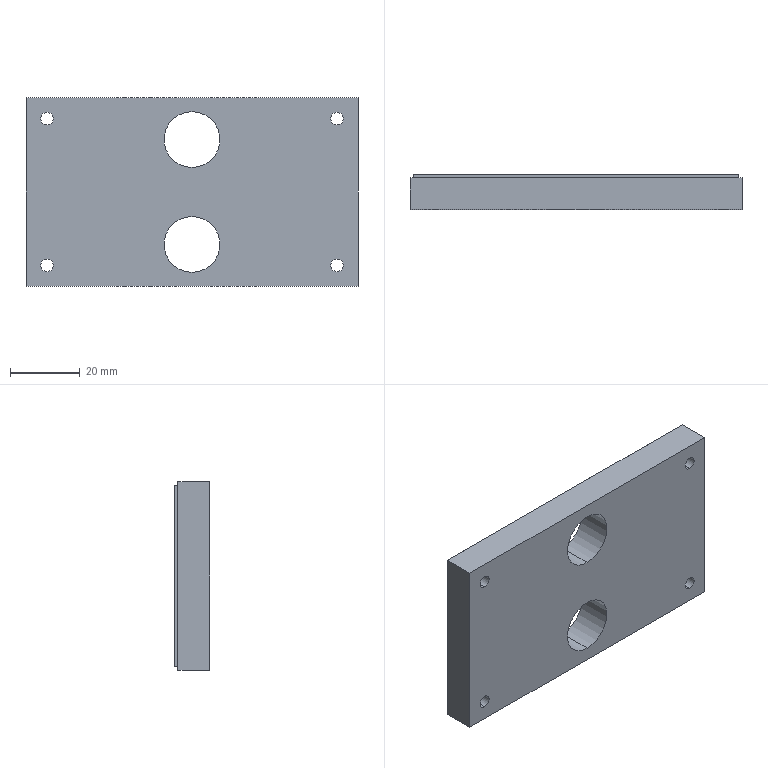Part | SolidWorks | features ICE 2, 3DProfileFeature 1, Chamfer 1, Extrusion 1, HoleWzd 1 | 1 solid | 43 faces | box 95 x 10.05 x 54 mm | volume 46492 mm3 | cylinder 20 | plane 15 | cone 8 | commonest cylinder face diameters 3.6 x8 7 x8 16 x4
STEP:
#1=CARTESIAN_POINT('',(47.5,0.,-4.));
#2=VERTEX_POINT('',#1);
#3=CARTESIAN_POINT('',(47.5,0.,-20.));
#4=VERTEX_POINT('',#3);
#5=CARTESIAN_POINT('',(47.5,0.,-12.));
#6=DIRECTION('',(0.,-1.,0.));
#7=DIRECTION('',(0.,0.,-1.));
#8=AXIS2_PLACEMENT_3D('',#5,#6,#7);
#9=CIRCLE('',#8,8.);
#10=EDGE_CURVE('',#2,#4,#9,.T.);
#11=ORIENTED_EDGE('',*,*,#10,.T.);
#12=CARTESIAN_POINT('',(47.5,10.05,-20.));
#13=VERTEX_POINT('',#12);
#14=CARTESIAN_POINT('',(47.5,-0.001,-20.));
#15=DIRECTION('',(0.,1.,0.));
#16=VECTOR('',#15,1000.);
#17=LINE('',#14,#16);
#18=EDGE_CURVE('',#4,#13,#17,.T.);
#19=ORIENTED_EDGE('',*,*,#18,.T.);
#20=CARTESIAN_POINT('',(47.5,10.05,-4.));
#21=VERTEX_POINT('',#20);
#22=CARTESIAN_POINT('',(47.5,10.05,-12.));
#23=DIRECTION('',(0.,-1.,0.));
#24=DIRECTION('',(0.,0.,1.));
#25=AXIS2_PLACEMENT_3D('',#22,#23,#24);
#26=CIRCLE('',#25,8.);
#27=EDGE_CURVE('',#21,#13,#26,.T.);
#28=ORIENTED_EDGE('',*,*,#27,.F.);
#29=CARTESIAN_POINT('',(47.5,-0.001,-4.));
#30=DIRECTION('',(0.,1.,0.));
#31=VECTOR('',#30,1000.);
#32=LINE('',#29,#31);
#33=EDGE_CURVE('',#2,#21,#32,.T.);
#34=ORIENTED_EDGE('',*,*,#33,.F.);
#35=EDGE_LOOP('',(#11,#19,#28,#34));
#36=FACE_OUTER_BOUND('',#35,.T.);
#37=CARTESIAN_POINT('',(47.5,-0.001,-12.));
#38=DIRECTION('',(0.,1.,0.));
#39=DIRECTION('',(0.,0.,1.));
#40=AXIS2_PLACEMENT_3D('',#37,#38,#39);
#41=CYLINDRICAL_SURFACE('',#40,8.);
#42=ADVANCED_FACE('',(#36),#41,.F.);
#43=CARTESIAN_POINT('',(47.5,0.,-50.));
#44=VERTEX_POINT('',#43);
#45=CARTESIAN_POINT('',(47.5,0.,-34.));
#46=VERTEX_POINT('',#45);
#47=CARTESIAN_POINT('',(47.5,0.,-42.));
#48=DIRECTION('',(0.,1.,0.));
#49=DIRECTION('',(0.,0.,-1.));
#50=AXIS2_PLACEMENT_3D('',#47,#48,#49);
#51=CIRCLE('',#50,8.);
#52=EDGE_CURVE('',#44,#46,#51,.T.);
#53=ORIENTED_EDGE('',*,*,#52,.F.);
#54=CARTESIAN_POINT('',(47.5,10.05,-50.));
#55=VERTEX_POINT('',#54);
#56=CARTESIAN_POINT('',(47.5,-0.001,-50.));
#57=DIRECTION('',(0.,1.,0.));
#58=VECTOR('',#57,1000.);
#59=LINE('',#56,#58);
#60=EDGE_CURVE('',#44,#55,#59,.T.);
#61=ORIENTED_EDGE('',*,*,#60,.T.);
#62=CARTESIAN_POINT('',(47.5,10.05,-34.));
#63=VERTEX_POINT('',#62);
#64=CARTESIAN_POINT('',(47.5,10.05,-42.));
#65=DIRECTION('',(0.,1.,0.));
#66=DIRECTION('',(0.,0.,1.));
#67=AXIS2_PLACEMENT_3D('',#64,#65,#66);
#68=CIRCLE('',#67,8.);
#69=EDGE_CURVE('',#55,#63,#68,.T.);
#70=ORIENTED_EDGE('',*,*,#69,.T.);
#71=CARTESIAN_POINT('',(47.5,-0.001,-34.));
#72=DIRECTION('',(0.,1.,0.));
#73=VECTOR('',#72,1000.);
#74=LINE('',#71,#73);
#75=EDGE_CURVE('',#46,#63,#74,.T.);
#76=ORIENTED_EDGE('',*,*,#75,.F.);
#77=EDGE_LOOP('',(#53,#61,#70,#76));
#78=FACE_OUTER_BOUND('',#77,.T.);
#79=CARTESIAN_POINT('',(47.5,-0.001,-42.));
#80=DIRECTION('',(0.,1.,0.));
#81=DIRECTION('',(0.,0.,1.));
#82=AXIS2_PLACEMENT_3D('',#79,#80,#81);
#83=CYLINDRICAL_SURFACE('',#82,8.);
#84=ADVANCED_FACE('',(#78),#83,.F.);
#85=CARTESIAN_POINT('',(6.,9.05,-51.5));
#86=VERTEX_POINT('',#85);
#87=CARTESIAN_POINT('',(6.,9.05,-44.5));
#88=VERTEX_POINT('',#87);
#89=CARTESIAN_POINT('',(6.,9.05,-48.));
#90=DIRECTION('',(0.,1.,0.));
#91=DIRECTION('',(0.,0.,-1.));
#92=AXIS2_PLACEMENT_3D('',#89,#90,#91);
#93=CIRCLE('',#92,3.5);
#94=EDGE_CURVE('',#86,#88,#93,.T.);
#95=ORIENTED_EDGE('',*,*,#94,.F.);
#96=CARTESIAN_POINT('',(6.,10.05,-52.5));
#97=VERTEX_POINT('',#96);
#98=CARTESIAN_POINT('',(6.,9.05,-51.5));
#99=DIRECTION('',(0.,0.7071,-0.7071));
#100=VECTOR('',#99,1000.);
#101=LINE('',#98,#100);
#102=EDGE_CURVE('',#86,#97,#101,.T.);
#103=ORIENTED_EDGE('',*,*,#102,.T.);
#104=CARTESIAN_POINT('',(6.,10.05,-43.5));
#105=VERTEX_POINT('',#104);
#106=CARTESIAN_POINT('',(6.,10.05,-48.));
#107=DIRECTION('',(0.,-1.,0.));
#108=DIRECTION('',(0.,0.,-1.));
#109=AXIS2_PLACEMENT_3D('',#106,#107,#108);
#110=CIRCLE('',#109,4.5);
#111=EDGE_CURVE('',#105,#97,#110,.T.);
#112=ORIENTED_EDGE('',*,*,#111,.F.);
#113=CARTESIAN_POINT('',(6.,9.05,-44.5));
#114=DIRECTION('',(0.,0.7071,0.7071));
#115=VECTOR('',#114,1000.);
#116=LINE('',#113,#115);
#117=EDGE_CURVE('',#88,#105,#116,.T.);
#118=ORIENTED_EDGE('',*,*,#117,.F.);
#119=EDGE_LOOP('',(#95,#103,#112,#118));
#120=FACE_OUTER_BOUND('',#119,.T.);
#121=CARTESIAN_POINT('',(6.,9.05,-48.));
#122=DIRECTION('',(0.,1.,0.));
#123=DIRECTION('',(0.,0.,1.));
#124=AXIS2_PLACEMENT_3D('',#121,#122,#123);
#125=CONICAL_SURFACE('',#124,3.5,0.7854);
#126=ADVANCED_FACE('',(#120),#125,.F.);
#127=CARTESIAN_POINT('',(6.,9.05,-9.5));
#128=VERTEX_POINT('',#127);
#129=CARTESIAN_POINT('',(6.,9.05,-2.5));
#130=VERTEX_POINT('',#129);
#131=CARTESIAN_POINT('',(6.,9.05,-6.));
#132=DIRECTION('',(0.,1.,0.));
#133=DIRECTION('',(0.,0.,-1.));
#134=AXIS2_PLACEMENT_3D('',#131,#132,#133);
#135=CIRCLE('',#134,3.5);
#136=EDGE_CURVE('',#128,#130,#135,.T.);
#137=ORIENTED_EDGE('',*,*,#136,.F.);
#138=CARTESIAN_POINT('',(6.,10.05,-10.5));
#139=VERTEX_POINT('',#138);
#140=CARTESIAN_POINT('',(6.,9.05,-9.5));
#141=DIRECTION('',(0.,0.7071,-0.7071));
#142=VECTOR('',#141,1000.);
#143=LINE('',#140,#142);
#144=EDGE_CURVE('',#128,#139,#143,.T.);
#145=ORIENTED_EDGE('',*,*,#144,.T.);
#146=CARTESIAN_POINT('',(6.,10.05,-1.5));
#147=VERTEX_POINT('',#146);
#148=CARTESIAN_POINT('',(6.,10.05,-6.));
#149=DIRECTION('',(0.,-1.,0.));
#150=DIRECTION('',(0.,0.,-1.));
#151=AXIS2_PLACEMENT_3D('',#148,#149,#150);
#152=CIRCLE('',#151,4.5);
#153=EDGE_CURVE('',#147,#139,#152,.T.);
#154=ORIENTED_EDGE('',*,*,#153,.F.);
#155=CARTESIAN_POINT('',(6.,9.05,-2.5));
#156=DIRECTION('',(0.,0.7071,0.7071));
#157=VECTOR('',#156,1000.);
#158=LINE('',#155,#157);
#159=EDGE_CURVE('',#130,#147,#158,.T.);
#160=ORIENTED_EDGE('',*,*,#159,.F.);
#161=EDGE_LOOP('',(#137,#145,#154,#160));
#162=FACE_OUTER_BOUND('',#161,.T.);
#163=CARTESIAN_POINT('',(6.,9.05,-6.));
#164=DIRECTION('',(0.,1.,0.));
#165=DIRECTION('',(0.,0.,1.));
#166=AXIS2_PLACEMENT_3D('',#163,#164,#165);
#167=CONICAL_SURFACE('',#166,3.5,0.7854);
#168=ADVANCED_FACE('',(#162),#167,.F.);
#169=CARTESIAN_POINT('',(89.,9.05,-51.5));
#170=VERTEX_POINT('',#169);
#171=CARTESIAN_POINT('',(89.,9.05,-44.5));
#172=VERTEX_POINT('',#171);
#173=CARTESIAN_POINT('',(89.,9.05,-48.));
#174=DIRECTION('',(0.,1.,0.));
#175=DIRECTION('',(0.,0.,-1.));
#176=AXIS2_PLACEMENT_3D('',#173,#174,#175);
#177=CIRCLE('',#176,3.5);
#178=EDGE_CURVE('',#170,#172,#177,.T.);
#179=ORIENTED_EDGE('',*,*,#178,.F.);
#180=CARTESIAN_POINT('',(89.,10.05,-52.5));
#181=VERTEX_POINT('',#180);
#182=CARTESIAN_POINT('',(89.,9.05,-51.5));
#183=DIRECTION('',(0.,0.7071,-0.7071));
#184=VECTOR('',#183,1000.);
#185=LINE('',#182,#184);
#186=EDGE_CURVE('',#170,#181,#185,.T.);
#187=ORIENTED_EDGE('',*,*,#186,.T.);
#188=CARTESIAN_POINT('',(89.,10.05,-43.5));
#189=VERTEX_POINT('',#188);
#190=CARTESIAN_POINT('',(89.,10.05,-48.));
#191=DIRECTION('',(0.,-1.,0.));
#192=DIRECTION('',(0.,0.,-1.));
#193=AXIS2_PLACEMENT_3D('',#190,#191,#192);
#194=CIRCLE('',#193,4.5);
#195=EDGE_CURVE('',#189,#181,#194,.T.);
#196=ORIENTED_EDGE('',*,*,#195,.F.);
#197=CARTESIAN_POINT('',(89.,9.05,-44.5));
#198=DIRECTION('',(0.,0.7071,0.7071));
#199=VECTOR('',#198,1000.);
#200=LINE('',#197,#199);
#201=EDGE_CURVE('',#172,#189,#200,.T.);
#202=ORIENTED_EDGE('',*,*,#201,.F.);
#203=EDGE_LOOP('',(#179,#187,#196,#202));
#204=FACE_OUTER_BOUND('',#203,.T.);
#205=CARTESIAN_POINT('',(89.,9.05,-48.));
#206=DIRECTION('',(0.,1.,0.));
#207=DIRECTION('',(0.,0.,1.));
#208=AXIS2_PLACEMENT_3D('',#205,#206,#207);
#209=CONICAL_SURFACE('',#208,3.5,0.7854);
#210=ADVANCED_FACE('',(#204),#209,.F.);
#211=CARTESIAN_POINT('',(89.,9.05,-9.5));
#212=VERTEX_POINT('',#211);
#213=CARTESIAN_POINT('',(89.,9.05,-2.5));
#214=VERTEX_POINT('',#213);
#215=CARTESIAN_POINT('',(89.,9.05,-6.));
#216=DIRECTION('',(0.,1.,0.));
#217=DIRECTION('',(0.,0.,-1.));
#218=AXIS2_PLACEMENT_3D('',#215,#216,#217);
#219=CIRCLE('',#218,3.5);
#220=EDGE_CURVE('',#212,#214,#219,.T.);
#221=ORIENTED_EDGE('',*,*,#220,.F.);
#222=CARTESIAN_POINT('',(89.,10.05,-10.5));
#223=VERTEX_POINT('',#222);
#224=CARTESIAN_POINT('',(89.,9.05,-9.5));
#225=DIRECTION('',(0.,0.7071,-0.7071));
#226=VECTOR('',#225,1000.);
#227=LINE('',#224,#226);
#228=EDGE_CURVE('',#212,#223,#227,.T.);
#229=ORIENTED_EDGE('',*,*,#228,.T.);
#230=CARTESIAN_POINT('',(89.,10.05,-1.5));
#231=VERTEX_POINT('',#230);
#232=CARTESIAN_POINT('',(89.,10.05,-6.));
#233=DIRECTION('',(0.,-1.,0.));
#234=DIRECTION('',(0.,0.,-1.));
#235=AXIS2_PLACEMENT_3D('',#232,#233,#234);
#236=CIRCLE('',#235,4.5);
#237=EDGE_CURVE('',#231,#223,#236,.T.);
#238=ORIENTED_EDGE('',*,*,#237,.F.);
#239=CARTESIAN_POINT('',(89.,9.05,-2.5));
#240=DIRECTION('',(0.,0.7071,0.7071));
#241=VECTOR('',#240,1000.);
#242=LINE('',#239,#241);
#243=EDGE_CURVE('',#214,#231,#242,.T.);
#244=ORIENTED_EDGE('',*,*,#243,.F.);
#245=EDGE_LOOP('',(#221,#229,#238,#244));
#246=FACE_OUTER_BOUND('',#245,.T.);
#247=CARTESIAN_POINT('',(89.,9.05,-6.));
#248=DIRECTION('',(0.,1.,0.));
#249=DIRECTION('',(0.,0.,1.));
#250=AXIS2_PLACEMENT_3D('',#247,#248,#249);
#251=CONICAL_SURFACE('',#250,3.5,0.7854);
#252=ADVANCED_FACE('',(#246),#251,.F.);
#253=CARTESIAN_POINT('',(6.,7.65,-51.5));
#254=VERTEX_POINT('',#253);
#255=CARTESIAN_POINT('',(6.,7.65,-44.5));
#256=VERTEX_POINT('',#255);
#257=CARTESIAN_POINT('',(6.,7.65,-48.));
#258=DIRECTION('',(0.,1.,0.));
#259=DIRECTION('',(0.,0.,1.));
#260=AXIS2_PLACEMENT_3D('',#257,#258,#259);
#261=CIRCLE('',#260,3.5);
#262=EDGE_CURVE('',#254,#256,#261,.T.);
#263=ORIENTED_EDGE('',*,*,#262,.F.);
#264=CARTESIAN_POINT('',(6.,10.05,-51.5));
#265=DIRECTION('',(0.,1.,0.));
#266=VECTOR('',#265,1000.);
#267=LINE('',#264,#266);
#268=EDGE_CURVE('',#254,#86,#267,.T.);
#269=ORIENTED_EDGE('',*,*,#268,.T.);
#270=ORIENTED_EDGE('',*,*,#94,.T.);
#271=CARTESIAN_POINT('',(6.,10.05,-44.5));
#272=DIRECTION('',(0.,1.,0.));
#273=VECTOR('',#272,1000.);
#274=LINE('',#271,#273);
#275=EDGE_CURVE('',#256,#88,#274,.T.);
#276=ORIENTED_EDGE('',*,*,#275,.F.);
#277=EDGE_LOOP('',(#263,#269,#270,#276));
#278=FACE_OUTER_BOUND('',#277,.T.);
#279=CARTESIAN_POINT('',(6.,10.05,-48.));
#280=DIRECTION('',(0.,1.,0.));
#281=DIRECTION('',(0.,0.,1.));
#282=AXIS2_PLACEMENT_3D('',#279,#280,#281);
#283=CYLINDRICAL_SURFACE('',#282,3.5);
#284=ADVANCED_FACE('',(#278),#283,.F.);
#285=CARTESIAN_POINT('',(6.,0.,-46.2));
#286=VERTEX_POINT('',#285);
#287=CARTESIAN_POINT('',(6.,0.,-49.8));
#288=VERTEX_POINT('',#287);
#289=CARTESIAN_POINT('',(6.,0.,-48.));
#290=DIRECTION('',(0.,-1.,0.));
#291=DIRECTION('',(0.,0.,-1.));
#292=AXIS2_PLACEMENT_3D('',#289,#290,#291);
#293=CIRCLE('',#292,1.8);
#294=EDGE_CURVE('',#286,#288,#293,.T.);
#295=ORIENTED_EDGE('',*,*,#294,.T.);
#296=CARTESIAN_POINT('',(6.,7.65,-49.8));
#297=VERTEX_POINT('',#296);
#298=CARTESIAN_POINT('',(6.,10.05,-49.8));
#299=DIRECTION('',(0.,1.,0.));
#300=VECTOR('',#299,1000.);
#301=LINE('',#298,#300);
#302=EDGE_CURVE('',#288,#297,#301,.T.);
#303=ORIENTED_EDGE('',*,*,#302,.T.);
#304=CARTESIAN_POINT('',(6.,7.65,-46.2));
#305=VERTEX_POINT('',#304);
#306=CARTESIAN_POINT('',(6.,7.65,-48.));
#307=DIRECTION('',(0.,1.,0.));
#308=DIRECTION('',(0.,0.,1.));
#309=AXIS2_PLACEMENT_3D('',#306,#307,#308);
#310=CIRCLE('',#309,1.8);
#311=EDGE_CURVE('',#297,#305,#310,.T.);
#312=ORIENTED_EDGE('',*,*,#311,.T.);
#313=CARTESIAN_POINT('',(6.,10.05,-46.2));
#314=DIRECTION('',(0.,1.,0.));
#315=VECTOR('',#314,1000.);
#316=LINE('',#313,#315);
#317=EDGE_CURVE('',#286,#305,#316,.T.);
#318=ORIENTED_EDGE('',*,*,#317,.F.);
#319=EDGE_LOOP('',(#295,#303,#312,#318));
#320=FACE_OUTER_BOUND('',#319,.T.);
#321=CARTESIAN_POINT('',(6.,10.05,-48.));
#322=DIRECTION('',(0.,1.,0.));
#323=DIRECTION('',(0.,0.,1.));
#324=AXIS2_PLACEMENT_3D('',#321,#322,#323);
#325=CYLINDRICAL_SURFACE('',#324,1.8);
#326=ADVANCED_FACE('',(#320),#325,.F.);
#327=CARTESIAN_POINT('',(89.,7.65,-51.5));
#328=VERTEX_POINT('',#327);
#329=CARTESIAN_POINT('',(89.,7.65,-44.5));
#330=VERTEX_POINT('',#329);
#331=CARTESIAN_POINT('',(89.,7.65,-48.));
#332=DIRECTION('',(0.,1.,0.));
#333=DIRECTION('',(0.,0.,1.));
#334=AXIS2_PLACEMENT_3D('',#331,#332,#333);
#335=CIRCLE('',#334,3.5);
#336=EDGE_CURVE('',#328,#330,#335,.T.);
#337=ORIENTED_EDGE('',*,*,#336,.F.);
#338=CARTESIAN_POINT('',(89.,10.05,-51.5));
#339=DIRECTION('',(0.,1.,0.));
#340=VECTOR('',#339,1000.);
#341=LINE('',#338,#340);
#342=EDGE_CURVE('',#328,#170,#341,.T.);
#343=ORIENTED_EDGE('',*,*,#342,.T.);
#344=ORIENTED_EDGE('',*,*,#178,.T.);
#345=CARTESIAN_POINT('',(89.,10.05,-44.5));
#346=DIRECTION('',(0.,1.,0.));
#347=VECTOR('',#346,1000.);
#348=LINE('',#345,#347);
#349=EDGE_CURVE('',#330,#172,#348,.T.);
#350=ORIENTED_EDGE('',*,*,#349,.F.);
#351=EDGE_LOOP('',(#337,#343,#344,#350));
#352=FACE_OUTER_BOUND('',#351,.T.);
#353=CARTESIAN_POINT('',(89.,10.05,-48.));
#354=DIRECTION('',(0.,1.,0.));
#355=DIRECTION('',(0.,0.,1.));
#356=AXIS2_PLACEMENT_3D('',#353,#354,#355);
#357=CYLINDRICAL_SURFACE('',#356,3.5);
#358=ADVANCED_FACE('',(#352),#357,.F.);
#359=CARTESIAN_POINT('',(89.,0.,-46.2));
#360=VERTEX_POINT('',#359);
#361=CARTESIAN_POINT('',(89.,0.,-49.8));
#362=VERTEX_POINT('',#361);
#363=CARTESIAN_POINT('',(89.,0.,-48.));
#364=DIRECTION('',(0.,-1.,0.));
#365=DIRECTION('',(0.,0.,-1.));
#366=AXIS2_PLACEMENT_3D('',#363,#364,#365);
#367=CIRCLE('',#366,1.8);
#368=EDGE_CURVE('',#360,#362,#367,.T.);
#369=ORIENTED_EDGE('',*,*,#368,.T.);
#370=CARTESIAN_POINT('',(89.,7.65,-49.8));
#371=VERTEX_POINT('',#370);
#372=CARTESIAN_POINT('',(89.,10.05,-49.8));
#373=DIRECTION('',(0.,1.,0.));
#374=VECTOR('',#373,1000.);
#375=LINE('',#372,#374);
#376=EDGE_CURVE('',#362,#371,#375,.T.);
#377=ORIENTED_EDGE('',*,*,#376,.T.);
#378=CARTESIAN_POINT('',(89.,7.65,-46.2));
#379=VERTEX_POINT('',#378);
#380=CARTESIAN_POINT('',(89.,7.65,-48.));
#381=DIRECTION('',(0.,1.,0.));
#382=DIRECTION('',(0.,0.,1.));
#383=AXIS2_PLACEMENT_3D('',#380,#381,#382);
#384=CIRCLE('',#383,1.8);
#385=EDGE_CURVE('',#371,#379,#384,.T.);
#386=ORIENTED_EDGE('',*,*,#385,.T.);
#387=CARTESIAN_POINT('',(89.,10.05,-46.2));
#388=DIRECTION('',(0.,1.,0.));
#389=VECTOR('',#388,1000.);
#390=LINE('',#387,#389);
#391=EDGE_CURVE('',#360,#379,#390,.T.);
#392=ORIENTED_EDGE('',*,*,#391,.F.);
#393=EDGE_LOOP('',(#369,#377,#386,#392));
#394=FACE_OUTER_BOUND('',#393,.T.);
#395=CARTESIAN_POINT('',(89.,10.05,-48.));
#396=DIRECTION('',(0.,1.,0.));
#397=DIRECTION('',(0.,0.,1.));
#398=AXIS2_PLACEMENT_3D('',#395,#396,#397);
#399=CYLINDRICAL_SURFACE('',#398,1.8);
#400=ADVANCED_FACE('',(#394),#399,.F.);
#401=CARTESIAN_POINT('',(89.,7.65,-9.5));
#402=VERTEX_POINT('',#401);
#403=CARTESIAN_POINT('',(89.,7.65,-2.5));
#404=VERTEX_POINT('',#403);
#405=CARTESIAN_POINT('',(89.,7.65,-6.));
#406=DIRECTION('',(0.,1.,0.));
#407=DIRECTION('',(0.,0.,1.));
#408=AXIS2_PLACEMENT_3D('',#405,#406,#407);
#409=CIRCLE('',#408,3.5);
#410=EDGE_CURVE('',#402,#404,#409,.T.);
#411=ORIENTED_EDGE('',*,*,#410,.F.);
#412=CARTESIAN_POINT('',(89.,10.05,-9.5));
#413=DIRECTION('',(0.,1.,0.));
#414=VECTOR('',#413,1000.);
#415=LINE('',#412,#414);
#416=EDGE_CURVE('',#402,#212,#415,.T.);
#417=ORIENTED_EDGE('',*,*,#416,.T.);
#418=ORIENTED_EDGE('',*,*,#220,.T.);
#419=CARTESIAN_POINT('',(89.,10.05,-2.5));
#420=DIRECTION('',(0.,1.,0.));
#421=VECTOR('',#420,1000.);
#422=LINE('',#419,#421);
#423=EDGE_CURVE('',#404,#214,#422,.T.);
#424=ORIENTED_EDGE('',*,*,#423,.F.);
#425=EDGE_LOOP('',(#411,#417,#418,#424));
#426=FACE_OUTER_BOUND('',#425,.T.);
#427=CARTESIAN_POINT('',(89.,10.05,-6.));
#428=DIRECTION('',(0.,1.,0.));
#429=DIRECTION('',(0.,0.,1.));
#430=AXIS2_PLACEMENT_3D('',#427,#428,#429);
#431=CYLINDRICAL_SURFACE('',#430,3.5);
#432=ADVANCED_FACE('',(#426),#431,.F.);
#433=CARTESIAN_POINT('',(89.,0.,-4.2));
#434=VERTEX_POINT('',#433);
#435=CARTESIAN_POINT('',(89.,0.,-7.8));
#436=VERTEX_POINT('',#435);
#437=CARTESIAN_POINT('',(89.,0.,-6.));
#438=DIRECTION('',(0.,-1.,0.));
#439=DIRECTION('',(0.,0.,-1.));
#440=AXIS2_PLACEMENT_3D('',#437,#438,#439);
#441=CIRCLE('',#440,1.8);
#442=EDGE_CURVE('',#434,#436,#441,.T.);
#443=ORIENTED_EDGE('',*,*,#442,.T.);
#444=CARTESIAN_POINT('',(89.,7.65,-7.8));
#445=VERTEX_POINT('',#444);
#446=CARTESIAN_POINT('',(89.,10.05,-7.8));
#447=DIRECTION('',(0.,1.,0.));
#448=VECTOR('',#447,1000.);
#449=LINE('',#446,#448);
#450=EDGE_CURVE('',#436,#445,#449,.T.);
#451=ORIENTED_EDGE('',*,*,#450,.T.);
#452=CARTESIAN_POINT('',(89.,7.65,-4.2));
#453=VERTEX_POINT('',#452);
#454=CARTESIAN_POINT('',(89.,7.65,-6.));
#455=DIRECTION('',(0.,1.,0.));
#456=DIRECTION('',(0.,0.,1.));
#457=AXIS2_PLACEMENT_3D('',#454,#455,#456);
#458=CIRCLE('',#457,1.8);
#459=EDGE_CURVE('',#445,#453,#458,.T.);
#460=ORIENTED_EDGE('',*,*,#459,.T.);
#461=CARTESIAN_POINT('',(89.,10.05,-4.2));
#462=DIRECTION('',(0.,1.,0.));
#463=VECTOR('',#462,1000.);
#464=LINE('',#461,#463);
#465=EDGE_CURVE('',#434,#453,#464,.T.);
#466=ORIENTED_EDGE('',*,*,#465,.F.);
#467=EDGE_LOOP('',(#443,#451,#460,#466));
#468=FACE_OUTER_BOUND('',#467,.T.);
#469=CARTESIAN_POINT('',(89.,10.05,-6.));
#470=DIRECTION('',(0.,1.,0.));
#471=DIRECTION('',(0.,0.,1.));
#472=AXIS2_PLACEMENT_3D('',#469,#470,#471);
#473=CYLINDRICAL_SURFACE('',#472,1.8);
#474=ADVANCED_FACE('',(#468),#473,.F.);
#475=CARTESIAN_POINT('',(6.,7.65,-9.5));
#476=VERTEX_POINT('',#475);
#477=CARTESIAN_POINT('',(6.,7.65,-2.5));
#478=VERTEX_POINT('',#477);
#479=CARTESIAN_POINT('',(6.,7.65,-6.));
#480=DIRECTION('',(0.,1.,0.));
#481=DIRECTION('',(0.,0.,1.));
#482=AXIS2_PLACEMENT_3D('',#479,#480,#481);
#483=CIRCLE('',#482,3.5);
#484=EDGE_CURVE('',#476,#478,#483,.T.);
#485=ORIENTED_EDGE('',*,*,#484,.F.);
#486=CARTESIAN_POINT('',(6.,10.05,-9.5));
#487=DIRECTION('',(0.,1.,0.));
#488=VECTOR('',#487,1000.);
#489=LINE('',#486,#488);
#490=EDGE_CURVE('',#476,#128,#489,.T.);
#491=ORIENTED_EDGE('',*,*,#490,.T.);
#492=ORIENTED_EDGE('',*,*,#136,.T.);
#493=CARTESIAN_POINT('',(6.,10.05,-2.5));
#494=DIRECTION('',(0.,1.,0.));
#495=VECTOR('',#494,1000.);
#496=LINE('',#493,#495);
#497=EDGE_CURVE('',#478,#130,#496,.T.);
#498=ORIENTED_EDGE('',*,*,#497,.F.);
#499=EDGE_LOOP('',(#485,#491,#492,#498));
#500=FACE_OUTER_BOUND('',#499,.T.);
#501=CARTESIAN_POINT('',(6.,10.05,-6.));
#502=DIRECTION('',(0.,1.,0.));
#503=DIRECTION('',(0.,0.,1.));
#504=AXIS2_PLACEMENT_3D('',#501,#502,#503);
#505=CYLINDRICAL_SURFACE('',#504,3.5);
#506=ADVANCED_FACE('',(#500),#505,.F.);
#507=CARTESIAN_POINT('',(6.,0.,-4.2));
#508=VERTEX_POINT('',#507);
#509=CARTESIAN_POINT('',(6.,0.,-7.8));
#510=VERTEX_POINT('',#509);
#511=CARTESIAN_POINT('',(6.,0.,-6.));
#512=DIRECTION('',(0.,-1.,0.));
#513=DIRECTION('',(0.,0.,-1.));
#514=AXIS2_PLACEMENT_3D('',#511,#512,#513);
#515=CIRCLE('',#514,1.8);
#516=EDGE_CURVE('',#508,#510,#515,.T.);
#517=ORIENTED_EDGE('',*,*,#516,.T.);
#518=CARTESIAN_POINT('',(6.,7.65,-7.8));
#519=VERTEX_POINT('',#518);
#520=CARTESIAN_POINT('',(6.,10.05,-7.8));
#521=DIRECTION('',(0.,1.,0.));
#522=VECTOR('',#521,1000.);
#523=LINE('',#520,#522);
#524=EDGE_CURVE('',#510,#519,#523,.T.);
#525=ORIENTED_EDGE('',*,*,#524,.T.);
#526=CARTESIAN_POINT('',(6.,7.65,-4.2));
#527=VERTEX_POINT('',#526);
#528=CARTESIAN_POINT('',(6.,7.65,-6.));
#529=DIRECTION('',(0.,1.,0.));
#530=DIRECTION('',(0.,0.,1.));
#531=AXIS2_PLACEMENT_3D('',#528,#529,#530);
#532=CIRCLE('',#531,1.8);
#533=EDGE_CURVE('',#519,#527,#532,.T.);
#534=ORIENTED_EDGE('',*,*,#533,.T.);
#535=CARTESIAN_POINT('',(6.,10.05,-4.2));
#536=DIRECTION('',(0.,1.,0.));
#537=VECTOR('',#536,1000.);
#538=LINE('',#535,#537);
#539=EDGE_CURVE('',#508,#527,#538,.T.);
#540=ORIENTED_EDGE('',*,*,#539,.F.);
#541=EDGE_LOOP('',(#517,#525,#534,#540));
#542=FACE_OUTER_BOUND('',#541,.T.);
#543=CARTESIAN_POINT('',(6.,10.05,-6.));
#544=DIRECTION('',(0.,1.,0.));
#545=DIRECTION('',(0.,0.,1.));
#546=AXIS2_PLACEMENT_3D('',#543,#544,#545);
#547=CYLINDRICAL_SURFACE('',#546,1.8);
#548=ADVANCED_FACE('',(#542),#547,.F.);
#549=CARTESIAN_POINT('',(0.,9.05,-54.));
#550=VERTEX_POINT('',#549);
#551=CARTESIAN_POINT('',(0.,9.05,0.));
#552=VERTEX_POINT('',#551);
#553=CARTESIAN_POINT('',(0.,9.05,0.));
#554=DIRECTION('',(0.,0.,1.));
#555=VECTOR('',#554,1000.);
#556=LINE('',#553,#555);
#557=EDGE_CURVE('',#550,#552,#556,.T.);
#558=ORIENTED_EDGE('',*,*,#557,.F.);
#559=CARTESIAN_POINT('',(0.,0.,-54.));
#560=VERTEX_POINT('',#559);
#561=CARTESIAN_POINT('',(0.,10.05,-54.));
#562=DIRECTION('',(0.,-1.,0.));
#563=VECTOR('',#562,1000.);
#564=LINE('',#561,#563);
#565=EDGE_CURVE('',#550,#560,#564,.T.);
#566=ORIENTED_EDGE('',*,*,#565,.T.);
#567=CARTESIAN_POINT('',(0.,0.,0.));
#568=VERTEX_POINT('',#567);
#569=CARTESIAN_POINT('',(0.,0.,0.));
#570=DIRECTION('',(0.,0.,1.));
#571=VECTOR('',#570,1000.);
#572=LINE('',#569,#571);
#573=EDGE_CURVE('',#560,#568,#572,.T.);
#574=ORIENTED_EDGE('',*,*,#573,.T.);
#575=CARTESIAN_POINT('',(0.,10.05,0.));
#576=DIRECTION('',(0.,-1.,0.));
#577=VECTOR('',#576,1000.);
#578=LINE('',#575,#577);
#579=EDGE_CURVE('',#552,#568,#578,.T.);
#580=ORIENTED_EDGE('',*,*,#579,.F.);
#581=EDGE_LOOP('',(#558,#566,#574,#580));
#582=FACE_OUTER_BOUND('',#581,.T.);
#583=CARTESIAN_POINT('',(0.,10.05,0.));
#584=DIRECTION('',(1.,0.,0.));
#585=DIRECTION('',(0.,0.,-1.));
#586=AXIS2_PLACEMENT_3D('',#583,#584,#585);
#587=PLANE('',#586);
#588=ADVANCED_FACE('',(#582),#587,.F.);
#589=CARTESIAN_POINT('',(95.,9.05,0.));
#590=VERTEX_POINT('',#589);
#591=CARTESIAN_POINT('',(0.,9.05,0.));
#592=DIRECTION('',(1.,0.,0.));
#593=VECTOR('',#592,1000.);
#594=LINE('',#591,#593);
#595=EDGE_CURVE('',#552,#590,#594,.T.);
#596=ORIENTED_EDGE('',*,*,#595,.F.);
#597=ORIENTED_EDGE('',*,*,#579,.T.);
#598=CARTESIAN_POINT('',(95.,0.,0.));
#599=VERTEX_POINT('',#598);
#600=CARTESIAN_POINT('',(0.,0.,0.));
#601=DIRECTION('',(1.,0.,0.));
#602=VECTOR('',#601,1000.);
#603=LINE('',#600,#602);
#604=EDGE_CURVE('',#568,#599,#603,.T.);
#605=ORIENTED_EDGE('',*,*,#604,.T.);
#606=CARTESIAN_POINT('',(95.,10.05,0.));
#607=DIRECTION('',(0.,-1.,0.));
#608=VECTOR('',#607,1000.);
#609=LINE('',#606,#608);
#610=EDGE_CURVE('',#590,#599,#609,.T.);
#611=ORIENTED_EDGE('',*,*,#610,.F.);
#612=EDGE_LOOP('',(#596,#597,#605,#611));
#613=FACE_OUTER_BOUND('',#612,.T.);
#614=CARTESIAN_POINT('',(0.,10.05,0.));
#615=DIRECTION('',(0.,0.,-1.));
#616=DIRECTION('',(-1.,0.,0.));
#617=AXIS2_PLACEMENT_3D('',#614,#615,#616);
#618=PLANE('',#617);
#619=ADVANCED_FACE('',(#613),#618,.F.);
#620=CARTESIAN_POINT('',(95.,9.05,-54.));
#621=VERTEX_POINT('',#620);
#622=CARTESIAN_POINT('',(95.,9.05,0.));
#623=DIRECTION('',(0.,0.,-1.));
#624=VECTOR('',#623,1000.);
#625=LINE('',#622,#624);
#626=EDGE_CURVE('',#590,#621,#625,.T.);
#627=ORIENTED_EDGE('',*,*,#626,.F.);
#628=ORIENTED_EDGE('',*,*,#610,.T.);
#629=CARTESIAN_POINT('',(95.,0.,-54.));
#630=VERTEX_POINT('',#629);
#631=CARTESIAN_POINT('',(95.,0.,0.));
#632=DIRECTION('',(0.,0.,-1.));
#633=VECTOR('',#632,1000.);
#634=LINE('',#631,#633);
#635=EDGE_CURVE('',#599,#630,#634,.T.);
#636=ORIENTED_EDGE('',*,*,#635,.T.);
#637=CARTESIAN_POINT('',(95.,10.05,-54.));
#638=DIRECTION('',(0.,-1.,0.));
#639=VECTOR('',#638,1000.);
#640=LINE('',#637,#639);
#641=EDGE_CURVE('',#621,#630,#640,.T.);
#642=ORIENTED_EDGE('',*,*,#641,.F.);
#643=EDGE_LOOP('',(#627,#628,#636,#642));
#644=FACE_OUTER_BOUND('',#643,.T.);
#645=CARTESIAN_POINT('',(95.,10.05,0.));
#646=DIRECTION('',(-1.,0.,0.));
#647=DIRECTION('',(0.,0.,1.));
#648=AXIS2_PLACEMENT_3D('',#645,#646,#647);
#649=PLANE('',#648);
#650=ADVANCED_FACE('',(#644),#649,.F.);
#651=CARTESIAN_POINT('',(0.,9.05,-54.));
#652=DIRECTION('',(-1.,0.,0.));
#653=VECTOR('',#652,1000.);
#654=LINE('',#651,#653);
#655=EDGE_CURVE('',#621,#550,#654,.T.);
#656=ORIENTED_EDGE('',*,*,#655,.F.);
#657=ORIENTED_EDGE('',*,*,#641,.T.);
#658=CARTESIAN_POINT('',(0.,0.,-54.));
#659=DIRECTION('',(-1.,0.,0.));
#660=VECTOR('',#659,1000.);
#661=LINE('',#658,#660);
#662=EDGE_CURVE('',#630,#560,#661,.T.);
#663=ORIENTED_EDGE('',*,*,#662,.T.);
#664=ORIENTED_EDGE('',*,*,#565,.F.);
#665=EDGE_LOOP('',(#656,#657,#663,#664));
#666=FACE_OUTER_BOUND('',#665,.T.);
#667=CARTESIAN_POINT('',(0.,10.05,-54.));
#668=DIRECTION('',(0.,0.,1.));
#669=DIRECTION('',(1.,0.,0.));
#670=AXIS2_PLACEMENT_3D('',#667,#668,#669);
#671=PLANE('',#670);
#672=ADVANCED_FACE('',(#666),#671,.F.);
#673=ORIENTED_EDGE('',*,*,#10,.F.);
#674=CARTESIAN_POINT('',(47.5,0.,-12.));
#675=DIRECTION('',(0.,-1.,0.));
#676=DIRECTION('',(0.,0.,-1.));
#677=AXIS2_PLACEMENT_3D('',#674,#675,#676);
#678=CIRCLE('',#677,8.);
#679=EDGE_CURVE('',#4,#2,#678,.T.);
#680=ORIENTED_EDGE('',*,*,#679,.F.);
#681=EDGE_LOOP('',(#673,#680));
#682=FACE_BOUND('',#681,.T.);
#683=CARTESIAN_POINT('',(47.5,0.,-42.));
#684=DIRECTION('',(0.,1.,0.));
#685=DIRECTION('',(0.,0.,-1.));
#686=AXIS2_PLACEMENT_3D('',#683,#684,#685);
#687=CIRCLE('',#686,8.);
#688=EDGE_CURVE('',#46,#44,#687,.T.);
#689=ORIENTED_EDGE('',*,*,#688,.T.);
#690=ORIENTED_EDGE('',*,*,#52,.T.);
#691=EDGE_LOOP('',(#689,#690));
#692=FACE_BOUND('',#691,.T.);
#693=ORIENTED_EDGE('',*,*,#294,.F.);
#694=CARTESIAN_POINT('',(6.,0.,-48.));
#695=DIRECTION('',(0.,-1.,0.));
#696=DIRECTION('',(0.,0.,-1.));
#697=AXIS2_PLACEMENT_3D('',#694,#695,#696);
#698=CIRCLE('',#697,1.8);
#699=EDGE_CURVE('',#288,#286,#698,.T.);
#700=ORIENTED_EDGE('',*,*,#699,.F.);
#701=EDGE_LOOP('',(#693,#700));
#702=FACE_BOUND('',#701,.T.);
#703=ORIENTED_EDGE('',*,*,#368,.F.);
#704=CARTESIAN_POINT('',(89.,0.,-48.));
#705=DIRECTION('',(0.,-1.,0.));
#706=DIRECTION('',(0.,0.,-1.));
#707=AXIS2_PLACEMENT_3D('',#704,#705,#706);
#708=CIRCLE('',#707,1.8);
#709=EDGE_CURVE('',#362,#360,#708,.T.);
#710=ORIENTED_EDGE('',*,*,#709,.F.);
#711=EDGE_LOOP('',(#703,#710));
#712=FACE_BOUND('',#711,.T.);
#713=ORIENTED_EDGE('',*,*,#442,.F.);
#714=CARTESIAN_POINT('',(89.,0.,-6.));
#715=DIRECTION('',(0.,-1.,0.));
#716=DIRECTION('',(0.,0.,-1.));
#717=AXIS2_PLACEMENT_3D('',#714,#715,#716);
#718=CIRCLE('',#717,1.8);
#719=EDGE_CURVE('',#436,#434,#718,.T.);
#720=ORIENTED_EDGE('',*,*,#719,.F.);
#721=EDGE_LOOP('',(#713,#720));
#722=FACE_BOUND('',#721,.T.);
#723=ORIENTED_EDGE('',*,*,#516,.F.);
#724=CARTESIAN_POINT('',(6.,0.,-6.));
#725=DIRECTION('',(0.,-1.,0.));
#726=DIRECTION('',(0.,0.,-1.));
#727=AXIS2_PLACEMENT_3D('',#724,#725,#726);
#728=CIRCLE('',#727,1.8);
#729=EDGE_CURVE('',#510,#508,#728,.T.);
#730=ORIENTED_EDGE('',*,*,#729,.F.);
#731=EDGE_LOOP('',(#723,#730));
#732=FACE_BOUND('',#731,.T.);
#733=ORIENTED_EDGE('',*,*,#573,.F.);
#734=ORIENTED_EDGE('',*,*,#662,.F.);
#735=ORIENTED_EDGE('',*,*,#635,.F.);
#736=ORIENTED_EDGE('',*,*,#604,.F.);
#737=EDGE_LOOP('',(#733,#734,#735,#736));
#738=FACE_OUTER_BOUND('',#737,.T.);
#739=CARTESIAN_POINT('',(0.,0.,0.));
#740=DIRECTION('',(0.,-1.,0.));
#741=DIRECTION('',(0.,0.,-1.));
#742=AXIS2_PLACEMENT_3D('',#739,#740,#741);
#743=PLANE('',#742);
#744=ADVANCED_FACE('',(#682,#692,#702,#712,#722,#732,#738),#743,.T.);
#745=CARTESIAN_POINT('',(94.,9.05,-1.));
#746=VERTEX_POINT('',#745);
#747=CARTESIAN_POINT('',(94.,9.05,-53.));
#748=VERTEX_POINT('',#747);
#749=CARTESIAN_POINT('',(94.,9.05,-1.));
#750=DIRECTION('',(0.,0.,-1.));
#751=VECTOR('',#750,1000.);
#752=LINE('',#749,#751);
#753=EDGE_CURVE('',#746,#748,#752,.T.);
#754=ORIENTED_EDGE('',*,*,#753,.F.);
#755=CARTESIAN_POINT('',(1.,9.05,-1.));
#756=VERTEX_POINT('',#755);
#757=CARTESIAN_POINT('',(1.,9.05,-1.));
#758=DIRECTION('',(1.,0.,0.));
#759=VECTOR('',#758,1000.);
#760=LINE('',#757,#759);
#761=EDGE_CURVE('',#756,#746,#760,.T.);
#762=ORIENTED_EDGE('',*,*,#761,.F.);
#763=CARTESIAN_POINT('',(1.,9.05,-53.));
#764=VERTEX_POINT('',#763);
#765=CARTESIAN_POINT('',(1.,9.05,-53.));
#766=DIRECTION('',(0.,0.,1.));
#767=VECTOR('',#766,1000.);
#768=LINE('',#765,#767);
#769=EDGE_CURVE('',#764,#756,#768,.T.);
#770=ORIENTED_EDGE('',*,*,#769,.F.);
#771=CARTESIAN_POINT('',(94.,9.05,-53.));
#772=DIRECTION('',(-1.,0.,0.));
#773=VECTOR('',#772,1000.);
#774=LINE('',#771,#773);
#775=EDGE_CURVE('',#748,#764,#774,.T.);
#776=ORIENTED_EDGE('',*,*,#775,.F.);
#777=EDGE_LOOP('',(#754,#762,#770,#776));
#778=FACE_BOUND('',#777,.T.);
#779=ORIENTED_EDGE('',*,*,#557,.T.);
#780=ORIENTED_EDGE('',*,*,#595,.T.);
#781=ORIENTED_EDGE('',*,*,#626,.T.);
#782=ORIENTED_EDGE('',*,*,#655,.T.);
#783=EDGE_LOOP('',(#779,#780,#781,#782));
#784=FACE_OUTER_BOUND('',#783,.T.);
#785=CARTESIAN_POINT('',(47.5,9.05,-27.));
#786=DIRECTION('',(0.,1.,0.));
#787=DIRECTION('',(0.,0.,1.));
#788=AXIS2_PLACEMENT_3D('',#785,#786,#787);
#789=PLANE('',#788);
#790=ADVANCED_FACE('',(#778,#784),#789,.T.);
#791=CARTESIAN_POINT('',(94.,10.05,-53.));
#792=VERTEX_POINT('',#791);
#793=CARTESIAN_POINT('',(1.,10.05,-53.));
#794=VERTEX_POINT('',#793);
#795=CARTESIAN_POINT('',(94.,10.05,-53.));
#796=DIRECTION('',(-1.,0.,0.));
#797=VECTOR('',#796,1000.);
#798=LINE('',#795,#797);
#799=EDGE_CURVE('',#792,#794,#798,.T.);
#800=ORIENTED_EDGE('',*,*,#799,.F.);
#801=CARTESIAN_POINT('',(94.,9.05,-53.));
#802=DIRECTION('',(0.,1.,0.));
#803=VECTOR('',#802,1000.);
#804=LINE('',#801,#803);
#805=EDGE_CURVE('',#748,#792,#804,.T.);
#806=ORIENTED_EDGE('',*,*,#805,.F.);
#807=ORIENTED_EDGE('',*,*,#775,.T.);
#808=CARTESIAN_POINT('',(1.,9.05,-53.));
#809=DIRECTION('',(0.,1.,0.));
#810=VECTOR('',#809,1000.);
#811=LINE('',#808,#810);
#812=EDGE_CURVE('',#764,#794,#811,.T.);
#813=ORIENTED_EDGE('',*,*,#812,.T.);
#814=EDGE_LOOP('',(#800,#806,#807,#813));
#815=FACE_OUTER_BOUND('',#814,.T.);
#816=CARTESIAN_POINT('',(94.,9.05,-53.));
#817=DIRECTION('',(0.,0.,-1.));
#818=DIRECTION('',(-1.,0.,0.));
#819=AXIS2_PLACEMENT_3D('',#816,#817,#818);
#820=PLANE('',#819);
#821=ADVANCED_FACE('',(#815),#820,.T.);
#822=CARTESIAN_POINT('',(94.,10.05,-1.));
#823=VERTEX_POINT('',#822);
#824=CARTESIAN_POINT('',(94.,10.05,-1.));
#825=DIRECTION('',(0.,0.,-1.));
#826=VECTOR('',#825,1000.);
#827=LINE('',#824,#826);
#828=EDGE_CURVE('',#823,#792,#827,.T.);
#829=ORIENTED_EDGE('',*,*,#828,.F.);
#830=CARTESIAN_POINT('',(94.,9.05,-1.));
#831=DIRECTION('',(0.,1.,0.));
#832=VECTOR('',#831,1000.);
#833=LINE('',#830,#832);
#834=EDGE_CURVE('',#746,#823,#833,.T.);
#835=ORIENTED_EDGE('',*,*,#834,.F.);
#836=ORIENTED_EDGE('',*,*,#753,.T.);
#837=ORIENTED_EDGE('',*,*,#805,.T.);
#838=EDGE_LOOP('',(#829,#835,#836,#837));
#839=FACE_OUTER_BOUND('',#838,.T.);
#840=CARTESIAN_POINT('',(94.,9.05,-1.));
#841=DIRECTION('',(1.,0.,0.));
#842=DIRECTION('',(0.,0.,-1.));
#843=AXIS2_PLACEMENT_3D('',#840,#841,#842);
#844=PLANE('',#843);
#845=ADVANCED_FACE('',(#839),#844,.T.);
#846=CARTESIAN_POINT('',(1.,10.05,-1.));
#847=VERTEX_POINT('',#846);
#848=CARTESIAN_POINT('',(1.,10.05,-1.));
#849=DIRECTION('',(1.,0.,0.));
#850=VECTOR('',#849,1000.);
#851=LINE('',#848,#850);
#852=EDGE_CURVE('',#847,#823,#851,.T.);
#853=ORIENTED_EDGE('',*,*,#852,.F.);
#854=CARTESIAN_POINT('',(1.,9.05,-1.));
#855=DIRECTION('',(0.,1.,0.));
#856=VECTOR('',#855,1000.);
#857=LINE('',#854,#856);
#858=EDGE_CURVE('',#756,#847,#857,.T.);
#859=ORIENTED_EDGE('',*,*,#858,.F.);
#860=ORIENTED_EDGE('',*,*,#761,.T.);
#861=ORIENTED_EDGE('',*,*,#834,.T.);
#862=EDGE_LOOP('',(#853,#859,#860,#861));
#863=FACE_OUTER_BOUND('',#862,.T.);
#864=CARTESIAN_POINT('',(1.,9.05,-1.));
#865=DIRECTION('',(0.,0.,1.));
#866=DIRECTION('',(1.,0.,0.));
#867=AXIS2_PLACEMENT_3D('',#864,#865,#866);
#868=PLANE('',#867);
#869=ADVANCED_FACE('',(#863),#868,.T.);
#870=CARTESIAN_POINT('',(1.,10.05,-53.));
#871=DIRECTION('',(0.,0.,1.));
#872=VECTOR('',#871,1000.);
#873=LINE('',#870,#872);
#874=EDGE_CURVE('',#794,#847,#873,.T.);
#875=ORIENTED_EDGE('',*,*,#874,.F.);
#876=ORIENTED_EDGE('',*,*,#812,.F.);
#877=ORIENTED_EDGE('',*,*,#769,.T.);
#878=ORIENTED_EDGE('',*,*,#858,.T.);
#879=EDGE_LOOP('',(#875,#876,#877,#878));
#880=FACE_OUTER_BOUND('',#879,.T.);
#881=CARTESIAN_POINT('',(1.,9.05,-53.));
#882=DIRECTION('',(-1.,0.,0.));
#883=DIRECTION('',(0.,0.,1.));
#884=AXIS2_PLACEMENT_3D('',#881,#882,#883);
#885=PLANE('',#884);
#886=ADVANCED_FACE('',(#880),#885,.T.);
#887=ORIENTED_EDGE('',*,*,#27,.T.);
#888=CARTESIAN_POINT('',(47.5,10.05,-12.));
#889=DIRECTION('',(0.,-1.,0.));
#890=DIRECTION('',(0.,0.,1.));
#891=AXIS2_PLACEMENT_3D('',#888,#889,#890);
#892=CIRCLE('',#891,8.);
#893=EDGE_CURVE('',#13,#21,#892,.T.);
#894=ORIENTED_EDGE('',*,*,#893,.T.);
#895=EDGE_LOOP('',(#887,#894));
#896=FACE_BOUND('',#895,.T.);
#897=CARTESIAN_POINT('',(47.5,10.05,-42.));
#898=DIRECTION('',(0.,1.,0.));
#899=DIRECTION('',(0.,0.,1.));
#900=AXIS2_PLACEMENT_3D('',#897,#898,#899);
#901=CIRCLE('',#900,8.);
#902=EDGE_CURVE('',#63,#55,#901,.T.);
#903=ORIENTED_EDGE('',*,*,#902,.F.);
#904=ORIENTED_EDGE('',*,*,#69,.F.);
#905=EDGE_LOOP('',(#903,#904));
#906=FACE_BOUND('',#905,.T.);
#907=ORIENTED_EDGE('',*,*,#237,.T.);
#908=CARTESIAN_POINT('',(89.,10.05,-6.));
#909=DIRECTION('',(0.,-1.,0.));
#910=DIRECTION('',(0.,0.,-1.));
#911=AXIS2_PLACEMENT_3D('',#908,#909,#910);
#912=CIRCLE('',#911,4.5);
#913=EDGE_CURVE('',#223,#231,#912,.T.);
#914=ORIENTED_EDGE('',*,*,#913,.T.);
#915=EDGE_LOOP('',(#907,#914));
#916=FACE_BOUND('',#915,.T.);
#917=ORIENTED_EDGE('',*,*,#195,.T.);
#918=CARTESIAN_POINT('',(89.,10.05,-48.));
#919=DIRECTION('',(0.,-1.,0.));
#920=DIRECTION('',(0.,0.,-1.));
#921=AXIS2_PLACEMENT_3D('',#918,#919,#920);
#922=CIRCLE('',#921,4.5);
#923=EDGE_CURVE('',#181,#189,#922,.T.);
#924=ORIENTED_EDGE('',*,*,#923,.T.);
#925=EDGE_LOOP('',(#917,#924));
#926=FACE_BOUND('',#925,.T.);
#927=ORIENTED_EDGE('',*,*,#153,.T.);
#928=CARTESIAN_POINT('',(6.,10.05,-6.));
#929=DIRECTION('',(0.,-1.,0.));
#930=DIRECTION('',(0.,0.,-1.));
#931=AXIS2_PLACEMENT_3D('',#928,#929,#930);
#932=CIRCLE('',#931,4.5);
#933=EDGE_CURVE('',#139,#147,#932,.T.);
#934=ORIENTED_EDGE('',*,*,#933,.T.);
#935=EDGE_LOOP('',(#927,#934));
#936=FACE_BOUND('',#935,.T.);
#937=ORIENTED_EDGE('',*,*,#111,.T.);
#938=CARTESIAN_POINT('',(6.,10.05,-48.));
#939=DIRECTION('',(0.,-1.,0.));
#940=DIRECTION('',(0.,0.,-1.));
#941=AXIS2_PLACEMENT_3D('',#938,#939,#940);
#942=CIRCLE('',#941,4.5);
#943=EDGE_CURVE('',#97,#105,#942,.T.);
#944=ORIENTED_EDGE('',*,*,#943,.T.);
#945=EDGE_LOOP('',(#937,#944));
#946=FACE_BOUND('',#945,.T.);
#947=ORIENTED_EDGE('',*,*,#799,.T.);
#948=ORIENTED_EDGE('',*,*,#874,.T.);
#949=ORIENTED_EDGE('',*,*,#852,.T.);
#950=ORIENTED_EDGE('',*,*,#828,.T.);
#951=EDGE_LOOP('',(#947,#948,#949,#950));
#952=FACE_OUTER_BOUND('',#951,.T.);
#953=CARTESIAN_POINT('',(0.,10.05,0.));
#954=DIRECTION('',(0.,-1.,0.));
#955=DIRECTION('',(0.,0.,-1.));
#956=AXIS2_PLACEMENT_3D('',#953,#954,#955);
#957=PLANE('',#956);
#958=ADVANCED_FACE('',(#896,#906,#916,#926,#936,#946,#952),#957,.F.);
#959=ORIENTED_EDGE('',*,*,#524,.F.);
#960=ORIENTED_EDGE('',*,*,#729,.T.);
#961=ORIENTED_EDGE('',*,*,#539,.T.);
#962=CARTESIAN_POINT('',(6.,7.65,-6.));
#963=DIRECTION('',(0.,1.,0.));
#964=DIRECTION('',(0.,0.,1.));
#965=AXIS2_PLACEMENT_3D('',#962,#963,#964);
#966=CIRCLE('',#965,1.8);
#967=EDGE_CURVE('',#527,#519,#966,.T.);
#968=ORIENTED_EDGE('',*,*,#967,.T.);
#969=EDGE_LOOP('',(#959,#960,#961,#968));
#970=FACE_OUTER_BOUND('',#969,.T.);
#971=CARTESIAN_POINT('',(6.,10.05,-6.));
#972=DIRECTION('',(0.,1.,0.));
#973=DIRECTION('',(0.,0.,1.));
#974=AXIS2_PLACEMENT_3D('',#971,#972,#973);
#975=CYLINDRICAL_SURFACE('',#974,1.8);
#976=ADVANCED_FACE('',(#970),#975,.F.);
#977=ORIENTED_EDGE('',*,*,#967,.F.);
#978=ORIENTED_EDGE('',*,*,#533,.F.);
#979=EDGE_LOOP('',(#977,#978));
#980=FACE_BOUND('',#979,.T.);
#981=CARTESIAN_POINT('',(6.,7.65,-6.));
#982=DIRECTION('',(0.,1.,0.));
#983=DIRECTION('',(0.,0.,1.));
#984=AXIS2_PLACEMENT_3D('',#981,#982,#983);
#985=CIRCLE('',#984,3.5);
#986=EDGE_CURVE('',#478,#476,#985,.T.);
#987=ORIENTED_EDGE('',*,*,#986,.T.);
#988=ORIENTED_EDGE('',*,*,#484,.T.);
#989=EDGE_LOOP('',(#987,#988));
#990=FACE_OUTER_BOUND('',#989,.T.);
#991=CARTESIAN_POINT('',(7.8,7.65,-6.));
#992=DIRECTION('',(0.,-1.,0.));
#993=DIRECTION('',(0.,0.,-1.));
#994=AXIS2_PLACEMENT_3D('',#991,#992,#993);
#995=PLANE('',#994);
#996=ADVANCED_FACE('',(#980,#990),#995,.F.);
#997=ORIENTED_EDGE('',*,*,#490,.F.);
#998=ORIENTED_EDGE('',*,*,#986,.F.);
#999=ORIENTED_EDGE('',*,*,#497,.T.);
#1000=CARTESIAN_POINT('',(6.,9.05,-6.));
#1001=DIRECTION('',(0.,1.,0.));
#1002=DIRECTION('',(0.,0.,-1.));
#1003=AXIS2_PLACEMENT_3D('',#1000,#1001,#1002);
#1004=CIRCLE('',#1003,3.5);
#1005=EDGE_CURVE('',#130,#128,#1004,.T.);
#1006=ORIENTED_EDGE('',*,*,#1005,.T.);
#1007=EDGE_LOOP('',(#997,#998,#999,#1006));
#1008=FACE_OUTER_BOUND('',#1007,.T.);
#1009=CARTESIAN_POINT('',(6.,10.05,-6.));
#1010=DIRECTION('',(0.,1.,0.));
#1011=DIRECTION('',(0.,0.,1.));
#1012=AXIS2_PLACEMENT_3D('',#1009,#1010,#1011);
#1013=CYLINDRICAL_SURFACE('',#1012,3.5);
#1014=ADVANCED_FACE('',(#1008),#1013,.F.);
#1015=ORIENTED_EDGE('',*,*,#450,.F.);
#1016=ORIENTED_EDGE('',*,*,#719,.T.);
#1017=ORIENTED_EDGE('',*,*,#465,.T.);
#1018=CARTESIAN_POINT('',(89.,7.65,-6.));
#1019=DIRECTION('',(0.,1.,0.));
#1020=DIRECTION('',(0.,0.,1.));
#1021=AXIS2_PLACEMENT_3D('',#1018,#1019,#1020);
#1022=CIRCLE('',#1021,1.8);
#1023=EDGE_CURVE('',#453,#445,#1022,.T.);
#1024=ORIENTED_EDGE('',*,*,#1023,.T.);
#1025=EDGE_LOOP('',(#1015,#1016,#1017,#1024));
#1026=FACE_OUTER_BOUND('',#1025,.T.);
#1027=CARTESIAN_POINT('',(89.,10.05,-6.));
#1028=DIRECTION('',(0.,1.,0.));
#1029=DIRECTION('',(0.,0.,1.));
#1030=AXIS2_PLACEMENT_3D('',#1027,#1028,#1029);
#1031=CYLINDRICAL_SURFACE('',#1030,1.8);
#1032=ADVANCED_FACE('',(#1026),#1031,.F.);
#1033=ORIENTED_EDGE('',*,*,#1023,.F.);
#1034=ORIENTED_EDGE('',*,*,#459,.F.);
#1035=EDGE_LOOP('',(#1033,#1034));
#1036=FACE_BOUND('',#1035,.T.);
#1037=CARTESIAN_POINT('',(89.,7.65,-6.));
#1038=DIRECTION('',(0.,1.,0.));
#1039=DIRECTION('',(0.,0.,1.));
#1040=AXIS2_PLACEMENT_3D('',#1037,#1038,#1039);
#1041=CIRCLE('',#1040,3.5);
#1042=EDGE_CURVE('',#404,#402,#1041,.T.);
#1043=ORIENTED_EDGE('',*,*,#1042,.T.);
#1044=ORIENTED_EDGE('',*,*,#410,.T.);
#1045=EDGE_LOOP('',(#1043,#1044));
#1046=FACE_OUTER_BOUND('',#1045,.T.);
#1047=CARTESIAN_POINT('',(90.8,7.65,-6.));
#1048=DIRECTION('',(0.,-1.,0.));
#1049=DIRECTION('',(0.,0.,-1.));
#1050=AXIS2_PLACEMENT_3D('',#1047,#1048,#1049);
#1051=PLANE('',#1050);
#1052=ADVANCED_FACE('',(#1036,#1046),#1051,.F.);
#1053=ORIENTED_EDGE('',*,*,#416,.F.);
#1054=ORIENTED_EDGE('',*,*,#1042,.F.);
#1055=ORIENTED_EDGE('',*,*,#423,.T.);
#1056=CARTESIAN_POINT('',(89.,9.05,-6.));
#1057=DIRECTION('',(0.,1.,0.));
#1058=DIRECTION('',(0.,0.,-1.));
#1059=AXIS2_PLACEMENT_3D('',#1056,#1057,#1058);
#1060=CIRCLE('',#1059,3.5);
#1061=EDGE_CURVE('',#214,#212,#1060,.T.);
#1062=ORIENTED_EDGE('',*,*,#1061,.T.);
#1063=EDGE_LOOP('',(#1053,#1054,#1055,#1062));
#1064=FACE_OUTER_BOUND('',#1063,.T.);
#1065=CARTESIAN_POINT('',(89.,10.05,-6.));
#1066=DIRECTION('',(0.,1.,0.));
#1067=DIRECTION('',(0.,0.,1.));
#1068=AXIS2_PLACEMENT_3D('',#1065,#1066,#1067);
#1069=CYLINDRICAL_SURFACE('',#1068,3.5);
#1070=ADVANCED_FACE('',(#1064),#1069,.F.);
#1071=ORIENTED_EDGE('',*,*,#376,.F.);
#1072=ORIENTED_EDGE('',*,*,#709,.T.);
#1073=ORIENTED_EDGE('',*,*,#391,.T.);
#1074=CARTESIAN_POINT('',(89.,7.65,-48.));
#1075=DIRECTION('',(0.,1.,0.));
#1076=DIRECTION('',(0.,0.,1.));
#1077=AXIS2_PLACEMENT_3D('',#1074,#1075,#1076);
#1078=CIRCLE('',#1077,1.8);
#1079=EDGE_CURVE('',#379,#371,#1078,.T.);
#1080=ORIENTED_EDGE('',*,*,#1079,.T.);
#1081=EDGE_LOOP('',(#1071,#1072,#1073,#1080));
#1082=FACE_OUTER_BOUND('',#1081,.T.);
#1083=CARTESIAN_POINT('',(89.,10.05,-48.));
#1084=DIRECTION('',(0.,1.,0.));
#1085=DIRECTION('',(0.,0.,1.));
#1086=AXIS2_PLACEMENT_3D('',#1083,#1084,#1085);
#1087=CYLINDRICAL_SURFACE('',#1086,1.8);
#1088=ADVANCED_FACE('',(#1082),#1087,.F.);
#1089=ORIENTED_EDGE('',*,*,#1079,.F.);
#1090=ORIENTED_EDGE('',*,*,#385,.F.);
#1091=EDGE_LOOP('',(#1089,#1090));
#1092=FACE_BOUND('',#1091,.T.);
#1093=CARTESIAN_POINT('',(89.,7.65,-48.));
#1094=DIRECTION('',(0.,1.,0.));
#1095=DIRECTION('',(0.,0.,1.));
#1096=AXIS2_PLACEMENT_3D('',#1093,#1094,#1095);
#1097=CIRCLE('',#1096,3.5);
#1098=EDGE_CURVE('',#330,#328,#1097,.T.);
#1099=ORIENTED_EDGE('',*,*,#1098,.T.);
#1100=ORIENTED_EDGE('',*,*,#336,.T.);
#1101=EDGE_LOOP('',(#1099,#1100));
#1102=FACE_OUTER_BOUND('',#1101,.T.);
#1103=CARTESIAN_POINT('',(90.8,7.65,-48.));
#1104=DIRECTION('',(0.,-1.,0.));
#1105=DIRECTION('',(0.,0.,-1.));
#1106=AXIS2_PLACEMENT_3D('',#1103,#1104,#1105);
#1107=PLANE('',#1106);
#1108=ADVANCED_FACE('',(#1092,#1102),#1107,.F.);
#1109=ORIENTED_EDGE('',*,*,#342,.F.);
#1110=ORIENTED_EDGE('',*,*,#1098,.F.);
#1111=ORIENTED_EDGE('',*,*,#349,.T.);
#1112=CARTESIAN_POINT('',(89.,9.05,-48.));
#1113=DIRECTION('',(0.,1.,0.));
#1114=DIRECTION('',(0.,0.,-1.));
#1115=AXIS2_PLACEMENT_3D('',#1112,#1113,#1114);
#1116=CIRCLE('',#1115,3.5);
#1117=EDGE_CURVE('',#172,#170,#1116,.T.);
#1118=ORIENTED_EDGE('',*,*,#1117,.T.);
#1119=EDGE_LOOP('',(#1109,#1110,#1111,#1118));
#1120=FACE_OUTER_BOUND('',#1119,.T.);
#1121=CARTESIAN_POINT('',(89.,10.05,-48.));
#1122=DIRECTION('',(0.,1.,0.));
#1123=DIRECTION('',(0.,0.,1.));
#1124=AXIS2_PLACEMENT_3D('',#1121,#1122,#1123);
#1125=CYLINDRICAL_SURFACE('',#1124,3.5);
#1126=ADVANCED_FACE('',(#1120),#1125,.F.);
#1127=ORIENTED_EDGE('',*,*,#302,.F.);
#1128=ORIENTED_EDGE('',*,*,#699,.T.);
#1129=ORIENTED_EDGE('',*,*,#317,.T.);
#1130=CARTESIAN_POINT('',(6.,7.65,-48.));
#1131=DIRECTION('',(0.,1.,0.));
#1132=DIRECTION('',(0.,0.,1.));
#1133=AXIS2_PLACEMENT_3D('',#1130,#1131,#1132);
#1134=CIRCLE('',#1133,1.8);
#1135=EDGE_CURVE('',#305,#297,#1134,.T.);
#1136=ORIENTED_EDGE('',*,*,#1135,.T.);
#1137=EDGE_LOOP('',(#1127,#1128,#1129,#1136));
#1138=FACE_OUTER_BOUND('',#1137,.T.);
#1139=CARTESIAN_POINT('',(6.,10.05,-48.));
#1140=DIRECTION('',(0.,1.,0.));
#1141=DIRECTION('',(0.,0.,1.));
#1142=AXIS2_PLACEMENT_3D('',#1139,#1140,#1141);
#1143=CYLINDRICAL_SURFACE('',#1142,1.8);
#1144=ADVANCED_FACE('',(#1138),#1143,.F.);
#1145=ORIENTED_EDGE('',*,*,#1135,.F.);
#1146=ORIENTED_EDGE('',*,*,#311,.F.);
#1147=EDGE_LOOP('',(#1145,#1146));
#1148=FACE_BOUND('',#1147,.T.);
#1149=CARTESIAN_POINT('',(6.,7.65,-48.));
#1150=DIRECTION('',(0.,1.,0.));
#1151=DIRECTION('',(0.,0.,1.));
#1152=AXIS2_PLACEMENT_3D('',#1149,#1150,#1151);
#1153=CIRCLE('',#1152,3.5);
#1154=EDGE_CURVE('',#256,#254,#1153,.T.);
#1155=ORIENTED_EDGE('',*,*,#1154,.T.);
#1156=ORIENTED_EDGE('',*,*,#262,.T.);
#1157=EDGE_LOOP('',(#1155,#1156));
#1158=FACE_OUTER_BOUND('',#1157,.T.);
#1159=CARTESIAN_POINT('',(7.8,7.65,-48.));
#1160=DIRECTION('',(0.,-1.,0.));
#1161=DIRECTION('',(0.,0.,-1.));
#1162=AXIS2_PLACEMENT_3D('',#1159,#1160,#1161);
#1163=PLANE('',#1162);
#1164=ADVANCED_FACE('',(#1148,#1158),#1163,.F.);
#1165=ORIENTED_EDGE('',*,*,#268,.F.);
#1166=ORIENTED_EDGE('',*,*,#1154,.F.);
#1167=ORIENTED_EDGE('',*,*,#275,.T.);
#1168=CARTESIAN_POINT('',(6.,9.05,-48.));
#1169=DIRECTION('',(0.,1.,0.));
#1170=DIRECTION('',(0.,0.,-1.));
#1171=AXIS2_PLACEMENT_3D('',#1168,#1169,#1170);
#1172=CIRCLE('',#1171,3.5);
#1173=EDGE_CURVE('',#88,#86,#1172,.T.);
#1174=ORIENTED_EDGE('',*,*,#1173,.T.);
#1175=EDGE_LOOP('',(#1165,#1166,#1167,#1174));
#1176=FACE_OUTER_BOUND('',#1175,.T.);
#1177=CARTESIAN_POINT('',(6.,10.05,-48.));
#1178=DIRECTION('',(0.,1.,0.));
#1179=DIRECTION('',(0.,0.,1.));
#1180=AXIS2_PLACEMENT_3D('',#1177,#1178,#1179);
#1181=CYLINDRICAL_SURFACE('',#1180,3.5);
#1182=ADVANCED_FACE('',(#1176),#1181,.F.);
#1183=ORIENTED_EDGE('',*,*,#228,.F.);
#1184=ORIENTED_EDGE('',*,*,#1061,.F.);
#1185=ORIENTED_EDGE('',*,*,#243,.T.);
#1186=ORIENTED_EDGE('',*,*,#913,.F.);
#1187=EDGE_LOOP('',(#1183,#1184,#1185,#1186));
#1188=FACE_OUTER_BOUND('',#1187,.T.);
#1189=CARTESIAN_POINT('',(89.,9.05,-6.));
#1190=DIRECTION('',(0.,1.,0.));
#1191=DIRECTION('',(0.,0.,1.));
#1192=AXIS2_PLACEMENT_3D('',#1189,#1190,#1191);
#1193=CONICAL_SURFACE('',#1192,3.5,0.7854);
#1194=ADVANCED_FACE('',(#1188),#1193,.F.);
#1195=ORIENTED_EDGE('',*,*,#186,.F.);
#1196=ORIENTED_EDGE('',*,*,#1117,.F.);
#1197=ORIENTED_EDGE('',*,*,#201,.T.);
#1198=ORIENTED_EDGE('',*,*,#923,.F.);
#1199=EDGE_LOOP('',(#1195,#1196,#1197,#1198));
#1200=FACE_OUTER_BOUND('',#1199,.T.);
#1201=CARTESIAN_POINT('',(89.,9.05,-48.));
#1202=DIRECTION('',(0.,1.,0.));
#1203=DIRECTION('',(0.,0.,1.));
#1204=AXIS2_PLACEMENT_3D('',#1201,#1202,#1203);
#1205=CONICAL_SURFACE('',#1204,3.5,0.7854);
#1206=ADVANCED_FACE('',(#1200),#1205,.F.);
#1207=ORIENTED_EDGE('',*,*,#144,.F.);
#1208=ORIENTED_EDGE('',*,*,#1005,.F.);
#1209=ORIENTED_EDGE('',*,*,#159,.T.);
#1210=ORIENTED_EDGE('',*,*,#933,.F.);
#1211=EDGE_LOOP('',(#1207,#1208,#1209,#1210));
#1212=FACE_OUTER_BOUND('',#1211,.T.);
#1213=CARTESIAN_POINT('',(6.,9.05,-6.));
#1214=DIRECTION('',(0.,1.,0.));
#1215=DIRECTION('',(0.,0.,1.));
#1216=AXIS2_PLACEMENT_3D('',#1213,#1214,#1215);
#1217=CONICAL_SURFACE('',#1216,3.5,0.7854);
#1218=ADVANCED_FACE('',(#1212),#1217,.F.);
#1219=ORIENTED_EDGE('',*,*,#102,.F.);
#1220=ORIENTED_EDGE('',*,*,#1173,.F.);
#1221=ORIENTED_EDGE('',*,*,#117,.T.);
#1222=ORIENTED_EDGE('',*,*,#943,.F.);
#1223=EDGE_LOOP('',(#1219,#1220,#1221,#1222));
#1224=FACE_OUTER_BOUND('',#1223,.T.);
#1225=CARTESIAN_POINT('',(6.,9.05,-48.));
#1226=DIRECTION('',(0.,1.,0.));
#1227=DIRECTION('',(0.,0.,1.));
#1228=AXIS2_PLACEMENT_3D('',#1225,#1226,#1227);
#1229=CONICAL_SURFACE('',#1228,3.5,0.7854);
#1230=ADVANCED_FACE('',(#1224),#1229,.F.);
#1231=ORIENTED_EDGE('',*,*,#60,.F.);
#1232=ORIENTED_EDGE('',*,*,#688,.F.);
#1233=ORIENTED_EDGE('',*,*,#75,.T.);
#1234=ORIENTED_EDGE('',*,*,#902,.T.);
#1235=EDGE_LOOP('',(#1231,#1232,#1233,#1234));
#1236=FACE_OUTER_BOUND('',#1235,.T.);
#1237=CARTESIAN_POINT('',(47.5,-0.001,-42.));
#1238=DIRECTION('',(0.,1.,0.));
#1239=DIRECTION('',(0.,0.,1.));
#1240=AXIS2_PLACEMENT_3D('',#1237,#1238,#1239);
#1241=CYLINDRICAL_SURFACE('',#1240,8.);
#1242=ADVANCED_FACE('',(#1236),#1241,.F.);
#1243=ORIENTED_EDGE('',*,*,#18,.F.);
#1244=ORIENTED_EDGE('',*,*,#679,.T.);
#1245=ORIENTED_EDGE('',*,*,#33,.T.);
#1246=ORIENTED_EDGE('',*,*,#893,.F.);
#1247=EDGE_LOOP('',(#1243,#1244,#1245,#1246));
#1248=FACE_OUTER_BOUND('',#1247,.T.);
#1249=CARTESIAN_POINT('',(47.5,-0.001,-12.));
#1250=DIRECTION('',(0.,1.,0.));
#1251=DIRECTION('',(0.,0.,1.));
#1252=AXIS2_PLACEMENT_3D('',#1249,#1250,#1251);
#1253=CYLINDRICAL_SURFACE('',#1252,8.);
#1254=ADVANCED_FACE('',(#1248),#1253,.F.);
#1255=CLOSED_SHELL('',(#42,#84,#126,#168,#210,#252,#284,#326,#358,#400,#432,#474,#506,#548,#588,#619,#650,#672,#744,#790,#821,#845,#869,#886,#958,#976,#996,#1014,#1032,#1052,#1070,#1088,#1108,#1126,#1144,#1164,#1182,#1194,#1206,#1218,#1230,#1242,#1254));
#1256=MANIFOLD_SOLID_BREP('',#1255);
#1257=CARTESIAN_POINT('',(0.,0.,0.));
#1258=DIRECTION('',(0.,0.,1.));
#1259=DIRECTION('',(1.,0.,0.));
#1260=AXIS2_PLACEMENT_3D('',#1257,#1258,#1259);
#1261=(LENGTH_UNIT()NAMED_UNIT(*)SI_UNIT(.MILLI.,.METRE.));
#1262=UNCERTAINTY_MEASURE_WITH_UNIT(LENGTH_MEASURE(0.00001),#1261,'','');
#1263=(NAMED_UNIT(*)PLANE_ANGLE_UNIT()SI_UNIT($,.RADIAN.));
#1264=(NAMED_UNIT(*)SI_UNIT($,.STERADIAN.)SOLID_ANGLE_UNIT());
#1265=(GEOMETRIC_REPRESENTATION_CONTEXT(3)GLOBAL_UNCERTAINTY_ASSIGNED_CONTEXT((#1262))GLOBAL_UNIT_ASSIGNED_CONTEXT((#1261,#1263,#1264))REPRESENTATION_CONTEXT('',''));
#1266=ADVANCED_BREP_SHAPE_REPRESENTATION('',(#1256,#1260),#1265);